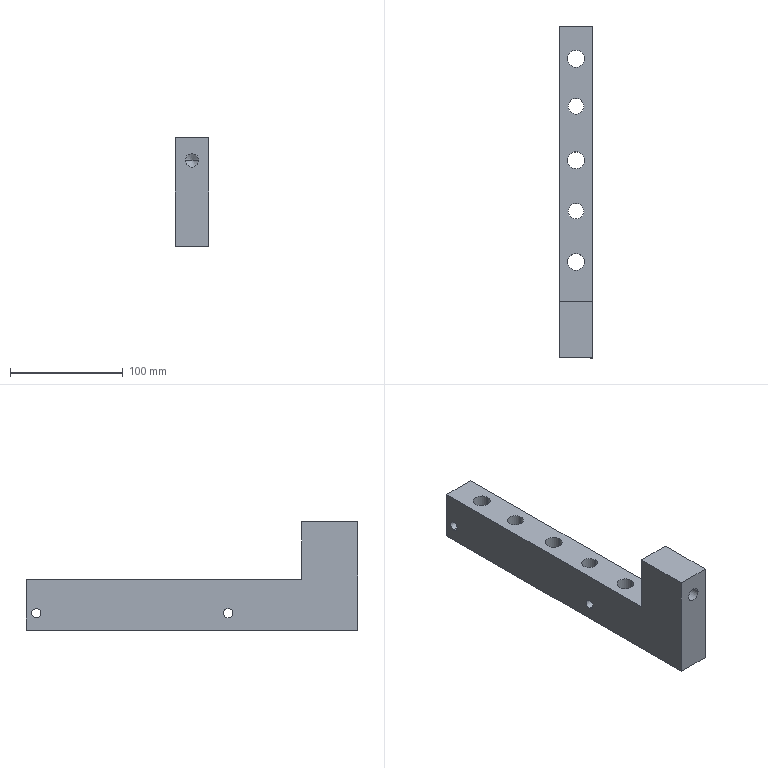Part | STEP file | THANH CHINH NGAM TRUOT 2_3 | 1 solid | 26 faces | box 30 x 294 x 96 mm | volume 428402 mm3 | cylinder 16 | plane 8 | cone 2 | commonest cylinder face diameters 15 x6 8.376 x4 14 x4 11.835 x2